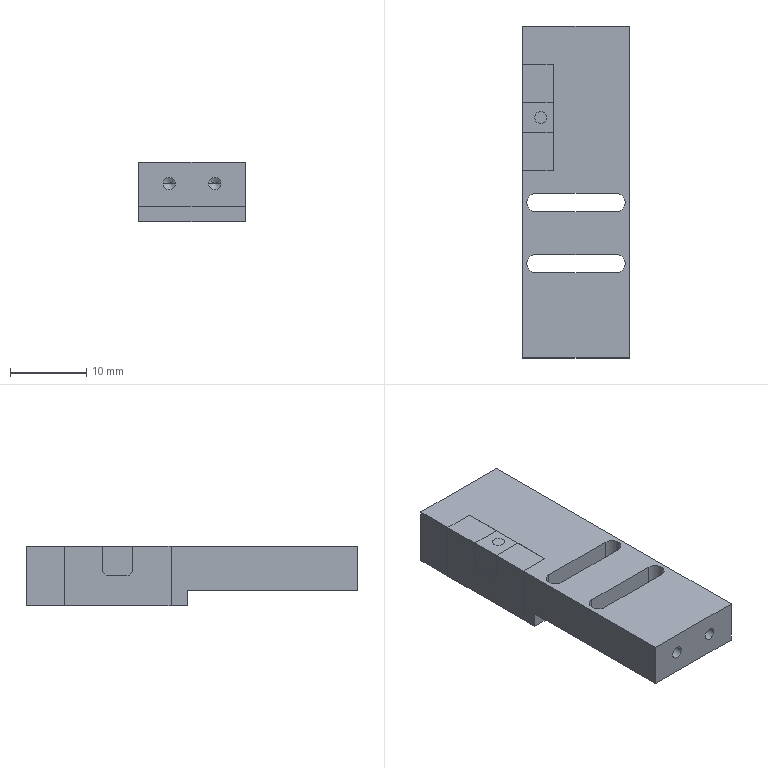CAM job | NX | 3+2 milling, drilling | part box 14 x 43.5 x 7.8 mm
Tools:
number,name,description,diameter,corner_radius,flute_length,length,flutes
9,D10JING,Milling Tool-5 Parameters,10.0,0.0,50.0,75.0,2
6,D6,Milling Tool-5 Parameters,6.0,0.0,50.0,75.0,2
10,D10,Milling Tool-5 Parameters,10.0,0.0,50.0,75.0,2
4,D4,Milling Tool-5 Parameters,4.0,0.0,50.0,75.0,2
13,D1.5,Milling Tool-5 Parameters,1.5,0.0,50.0,75.0,2
7,D6A45,Milling Tool-5 Parameters,6.0,0.0,50.0,75.0,2
14,1.6ZT,Drilling Tool,1.6,0.0,35.0,50.0,2
Operations:
program,operation,operation_type,tool,method,geometry_group,spindle_rpm,surface_speed,feed_per_tooth,feed_cut,feed_plunge,cut_length_mm,path_length_mm,cut_time_min,machine_time_min
1,FLOOR_WALL,VolumeBased25DMillingOperation,D10JING,METHOD,A,9500.0,298.0,0.0658,1250.0,100.0,255.997,309.997,0.2048,0.2102
1,DRILLING_COPY_1,Operation,D6A45,METHOD,A,5000.0,94.0,0.025,250.0,0.0,8.0,94.474,0.032,0.0406
1,DRILLING_COPY_COPY_COPY,Operation,1.6ZT,METHOD,A,2000.0,20.0,0.0375,150.0,0.0,22.261,122.996,0.1484,0.1585
1,ZLEVEL_PROFILE,ZLevelMilling,D10,METHOD,A,9500.0,298.0,0.1316,2500.0,1000.0,2419.459,2484.109,0.9905,0.9969
1,FLOOR_WALL_1,VolumeBased25DMillingOperation,D6,METHOD,A,9500.0,179.0,0.1316,2500.0,1000.0,566.24,656.649,0.2409,0.2499
1,FLOOR_WALL_1_COPY,VolumeBased25DMillingOperation,D6,METHOD,A,9500.0,179.0,0.0632,1200.0,1000.0,211.057,273.357,0.1769,0.1831
1,ZLEVEL_PROFILE_COPY_COPY_COPY,ZLevelMilling,D1.5,METHOD,A,9500.0,44.0,0.0526,1000.0,1000.0,2839.683,2982.197,2.84,2.854
1,HOLE_MILLING,CylinderMilling,D1.5,METHOD,A,9500.0,44.0,0.0447,850.0,100.0,58.166,125.366,0.0684,0.0752
1,PLANAR_MILL_COPY_1_COPY,PlanarMilling,D6A45,METHOD,A,9500.0,179.0,0.0658,1250.0,100.0,82.134,141.134,0.0657,0.0716
1,PLANAR_MILL_COPY_1_COPY_COPY,PlanarMilling,D6A45,METHOD,A,9500.0,179.0,0.0658,1250.0,100.0,99.511,301.647,0.0796,0.0998
1,CUT_COMP,CylinderMilling,D1.5,METHOD,A,9500.0,44.0,0.0447,850.0,100.0,16.451,83.651,0.0194,0.0261
1,111,ZLevelMilling,D6,METHOD,A,9500.0,298.0,0.0632,1200.0,1000.0,142.805,214.105,0.1197,0.1269
2,DRILLING,Operation,D6A45,METHOD,B,5000.0,94.0,0.025,250.0,0.0,16.0,119.929,0.064,0.0744
2,DRILLING_COPY_COPY,Operation,1.6ZT,METHOD,B,2000.0,20.0,0.0375,150.0,0.0,30.56,149.048,0.2037,0.2156
2,HOLE_MILLING_COPY,CylinderMilling,D1.5,METHOD,B,9500.0,44.0,0.0447,850.0,100.0,130.499,262.097,0.1535,0.1667
2,DRILLING_COPY,Operation,D6A45,METHOD,B,5000.0,94.0,0.025,250.0,0.0,8.3,84.6,0.0332,0.0408
2,CUT_COMP_COPY,CylinderMilling,D1.5,METHOD,B,9500.0,44.0,0.0447,850.0,100.0,36.495,168.093,0.0429,0.0561
3,DRILLING_COPY_1_COPY,Operation,D6A45,METHOD,C,5000.0,94.0,0.025,250.0,0.0,8.0,88.487,0.032,0.04
3,DRILLING_COPY_COPY_COPY_COPY,Operation,1.6ZT,METHOD,C,2000.0,20.0,0.0375,150.0,0.0,25.361,123.21,0.1691,0.1789
3,FLOOR_WALL_1_COPY_1,VolumeBased25DMillingOperation,D4,METHOD,C,9500.0,179.0,0.1316,2500.0,1000.0,549.73,615.53,0.2499,0.2565
3,FLOOR_WALL_1_COPY_COPY,VolumeBased25DMillingOperation,D4,METHOD,C,9500.0,179.0,0.0632,1200.0,1000.0,130.22,196.421,0.1103,0.1169
3,PLANAR_MILL_COPY_1_COPY_COPY_1,PlanarMilling,D6A45,METHOD,C,9500.0,179.0,0.0658,1250.0,100.0,49.335,108.335,0.0395,0.0454
3,CUT_COMP4,VolumeBased25DMillingOperation,D4,METHOD,C,9500.0,179.0,0.0632,1200.0,1000.0,49.838,115.838,0.0428,0.0494